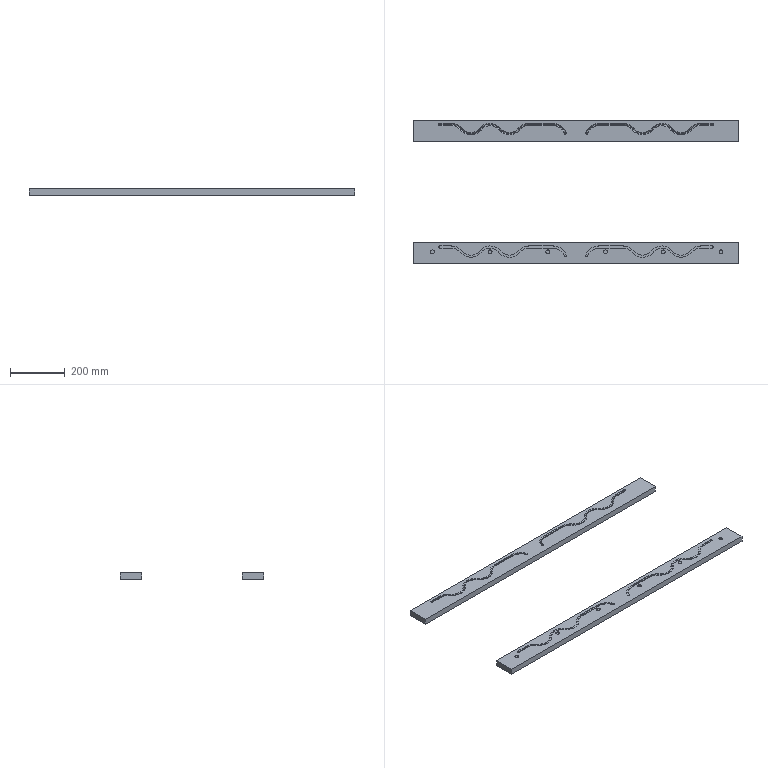CAM job | NX | 3-axis milling, drilling | part box 1185 x 523.484 x 22 mm | stock box 1185 x 523.484 x 22 mm
Tools:
number,name,description,diameter,corner_radius,flute_length,length,flutes
0,D6点孔钻,Drilling Tool,10.0,0.0,5.0,40.0,2
0,Z10.3钻头,Drilling Tool,10.2,0.0,35.0,50.0,2
0,Z4.2钻头,Drilling Tool,4.0,0.0,35.0,50.0,2
0,D3平底刀,Milling Tool-5 Parameters,3.0,0.2,8.0,8.0,3
0,R2球刀,Milling Tool-5 Parameters,4.0,2.0,4.0,20.0,2
Operations:
program,operation,operation_type,tool,method,geometry_group,spindle_rpm,surface_speed,feed_per_tooth,feed_cut,feed_plunge,cut_length_mm,path_length_mm,cut_time_min,machine_time_min
0126.NC,G81点孔,Operation,D6点孔钻,METHOD,WORKPIECE---A,1500.0,47.0,0.04,120.0,0.0,18.0,1193.527,0.15,0.2676
0126.NC,G83钻孔,Operation,Z10.3钻头,METHOD,WORKPIECE---A,800.0,25.0,0.05,80.0,0.0,129.0,1415.527,1.613,1.741
0126.NC,G83钻孔_1,Operation,Z4.2钻头,METHOD,WORKPIECE---A,1000.0,12.0,0.01,20.0,0.0,26.0,1061.511,1.3,1.404
0127.NC,PLANAR_PROFILE,PlanarMilling,R2球刀,METHOD,WORKPIECE---A,3000.0,37.0,0.3333,2000.0,100.0,42401.563,50965.162,21.201,22.057
0127.NC,定轴曲面加工,SurfaceContour,D3平底刀,METHOD,WORKPIECE---A,3000.0,28.0,0.3889,3500.0,70.0,83835.204,88608.673,23.962,24.439